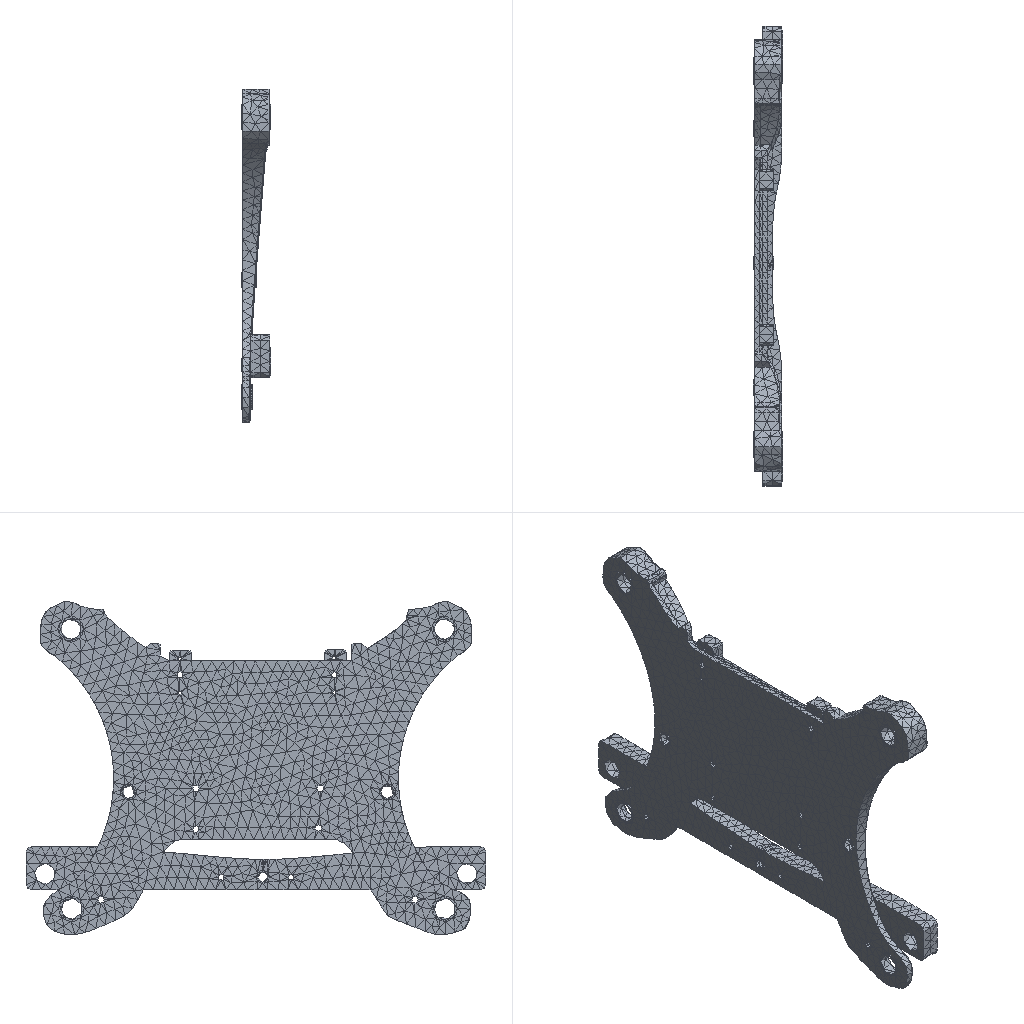Simulation study | ansys workbench
Ansys APDL input file, long lists of numbers shortened:
/batch
/config,noeldb,1     ! force off writing results to database
*get,_wallstrt,active,,time,wall
! ANSYS input file written by Workbench version 2022 R2
! File used for geometry attach:
/title,_____--__ (B5)
! ****** Begin Custom Load Command Snippet ******
/COM, ACT Extensions:
/COM,     LSDYNA, 2022.2
/COM,/COM,     ANSYSMotion, 2022.2
/COM,
! ****** End   Custom Load Command Snippet ******
*DIM,_wb_ProjectScratch_dir,string,248
_wb_ProjectScratch_dir(1) = ''
*DIM,_wb_SolverFiles_dir,string,248
_wb_SolverFiles_dir(1) = ''
*DIM,_wb_userfiles_dir,string,248
_wb_userfiles_dir(1) = ''
/com,--- Data in consistent NMM units. See Solving Units in the help system for more information.
/units,MPA
/nopr
/wb,file,start              !  signify a WB generated input file
/prep7
! Turn off shape checking because checks already performed inside WB mesher.
! See help system for more information.
SHPP,OFF,,NOWARN
/nolist
etcon,set             ! allow ANSYS to choose best KEYOP's for 180x elements, resets any applicable keyopt to MAPDL defaults
/com,*********** Nodes for the whole assembly ***********
nblock,3,,33969
(1i9,3e20.9e3)
        1     3.263410559E+01     3.933549495E+02    -1.201904341E+02
! (30880 more lines like these left out)
-1
/wb,elem,start            !  set before creation of elements
/com,*********** Elements for Body 1 "_____(2)-FreeParts|_____(2)" ***********
et,1,187
eblock,19,solid,,16207
(19i9)
        1        1        1        1        0        0        0        0       10        0        1      141     2428     2638     4977     6172    21111     6173     6178
! (32413 more lines like these left out)
-1
/wb,elem,end               !  done creating elements
/com,*********** Send User Defined Coordinate System(s) ***********
csys,0
toffst,273.15,  ! Temperature offset from absolute zero
/com,*********** Set Reference Temperature ***********
tref,22.
/wb,mat,start              !  starting to send materials
/com,*********** Send Materials ***********
MP,DENS,1,7.85e-09,	! tonne mm^-3
MP,EX,1,210000,	! tonne s^-2 mm^-1
MP,NUXY,1,0.3,
/wb,mat,end                !  done sending materials
!************************* Model Summary ********************
!_____(2)-FreeParts|_____(2),	热扎酸洗高强度钢,	matid,	1
!************************* End Model Summary ********************
! get the diagonal of the bounding box. Needed later for other things
*get,_xmin,node,,mnloc,x
*get,_ymin,node,,mnloc,y
*get,_zmin,node,,mnloc,z
*get,_xmax,node,,mxloc,x
*get,_ymax,node,,mxloc,y
*get,_zmax,node,,mxloc,z
_ASMDIAG=(_xmax-_xmin)*(_xmax-_xmin)+(_ymax-_ymin)*(_ymax-_ymin)+(_zmax-_zmin)*(_zmax-_zmin)
_ASMDIAG=SQRT(_ASMDIAG)
/wb,contact,start          !  starting to send contact
/wb,contact,end            !  done creating contacts
/golist
/wb,load,start             !  starting to send loads
/com,*********** Fixed Supports ***********
CMBLOCK,_FIXEDSU,NODE,      341
(8i10)
      2177      2178      2179      2180      2181      2182      2183      2192
! (42 more lines like these left out)
cmsel,s,_FIXEDSU
d,all,all
nsel,all
/gst,on,on
fini
*get,_numnode,node,0,count
*get,_numelem,elem,0,count
*get, _MAXELEMNUM, elem, 0, NUM, MAX
*get, _MAXNODENUM, node, 0, NUM, MAX
*get, _MAXELEMTYPE, etyp, 0, NUM, MAX
*get, _MAXREALCONST, rcon, 0, NUM, MAX
/go
/wb,load,end               !  done creating loads
/com,--- Number of total nodes = %_numnode%
/com,--- Number of contact elements = 0
/com,--- Number of spring elements = 0
/com,--- Number of bearing elements = 0
/com,--- Number of solid elements = 16207
/com,--- Number of condensed parts = 0
/com,--- Number of total elements = %_numelem%
*get,_wallbsol,active,,time,wall
/solu
antype,2                   ! modal analysis
_thickRatio=  1     ! Ratio of thick parts in the model
modopt,lanb,6
outres,erase
outres,all,none
outres,nsol,all
mxpand                    ! default expand in case of complex solution
dmpopt,esav,no
dmpopt,emat,no
dmpopt,full,no
! *********** WB SOLVE COMMAND ***********
! check interactive state
*get,ANSINTER_,active,,int
*if,ANSINTER_,ne,0,then
/eof
*endif
solve
/com *************** Write FE CONNECTORS *********
CEWRITE,file,ce,,INTE
*get,_nmodalsolproc,active,0,numcpu
fini
/nopr
*get,_numnode,node,0,count
*get,_numelem,elem,0,count
*get, _MAXELEMNUM, elem, 0, NUM, MAX
*get, _MAXNODENUM, node, 0, NUM, MAX,,,INTERNAL
*get, _MAXELEMTYPE, etyp, 0, NUM, MAX
*get, _MAXREALCONST, rcon, 0, NUM, MAX
*get,_NSOLTHREADS,active,0,ntfs
*get,_NSOLPROCESSES,active,0,npfs
/gopr
*get,_wallasol,active,,time,wall
/post1
/nopr
*dim,_direction,CHAR,6,1
_direction(1) = 'X'
_direction(2) = 'Y'
_direction(3) = 'Z'
_direction(4) = 'ROTX'
_direction(5) = 'ROTY'
_direction(6) = 'ROTZ'
*get,_lastLS,active,0,set,LSTP
*get,_beginset,active,0,set,nset,first,_lastLS
*get,_endset,active,0,set,nset,last,_lastLS
_nummodes = 0
*if,_endset,gt,0,then
_nummodes = _endset - _beginset + 1
*endif
*do,i_mode,1,_nummodes
   *do,j_component,1,6
			*get,PFACT_%i_mode%_%j_component%,MODE,%i_mode%,PFACT,,DIREC,_direction(%j_component%)
   *enddo
*enddo
*dim,_tmdirection,CHAR,6,1
_tmdirection(1) = 'X'
_tmdirection(2) = 'Y'
_tmdirection(3) = 'Z'
_tmdirection(4) = 'X'
_tmdirection(5) = 'Y'
_tmdirection(6) = 'Z'
*do,j_component,1,6
    *if,j_component,gt,3,then
        *get,TOTALMASS_%j_component%,ELEM,0,IOR,_tmdirection(%j_component%)
    *else
        *get,TOTALMASS_%j_component%,ELEM,0,MTOT,_tmdirection(%j_component%)
    *endif
*enddo
/gopr
xmlo,ENCODING,ISO-8859-1
xmlo,parm
/xml,parm,xml
fini
/gopr
*get,_walldone,active,,time,wall
_preptime=(_wallbsol-_wallstrt)*3600
_solvtime=(_wallasol-_wallbsol)*3600
_posttime=(_walldone-_wallasol)*3600
_totaltim=(_walldone-_wallstrt)*3600
*get,_dlbratio,active,0,solu,dlbr
*get,_combtime,active,0,solu,comb
*get,_ssmode,active,0,solu,ssmm
*get,_ndofs,active,0,solu,ndof
/fclean				!clean distributed files
/com,--- Total number of nodes = %_numnode%
/com,--- Total number of elements = %_numelem%
/com,--- Element load balance ratio = %_dlbratio%
/com,--- Time to combine distributed files = %_combtime%
/com,--- Sparse memory mode = %_ssmode%
/com,--- Number of DOF = %_ndofs%
/wb,file,end               ! done with WB generated input